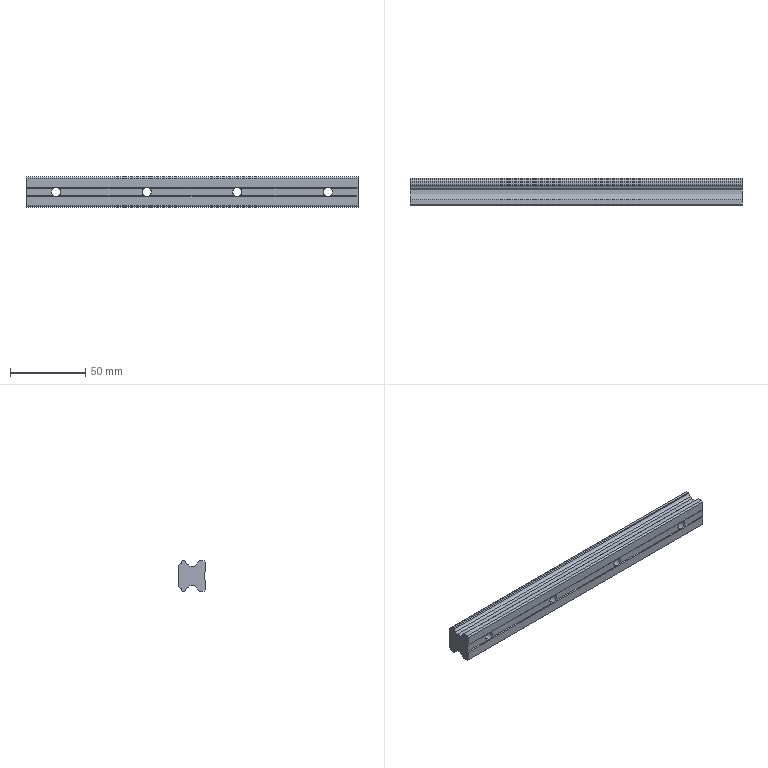Part | SolidWorks | features BaseBody 1 | 1 solid | 62 faces | box 220 x 18 x 20 mm | volume 62917 mm3 | plane 42 | cylinder 20 | commonest cylinder face diameters 6 x8 9.5 x8 4.12 x4